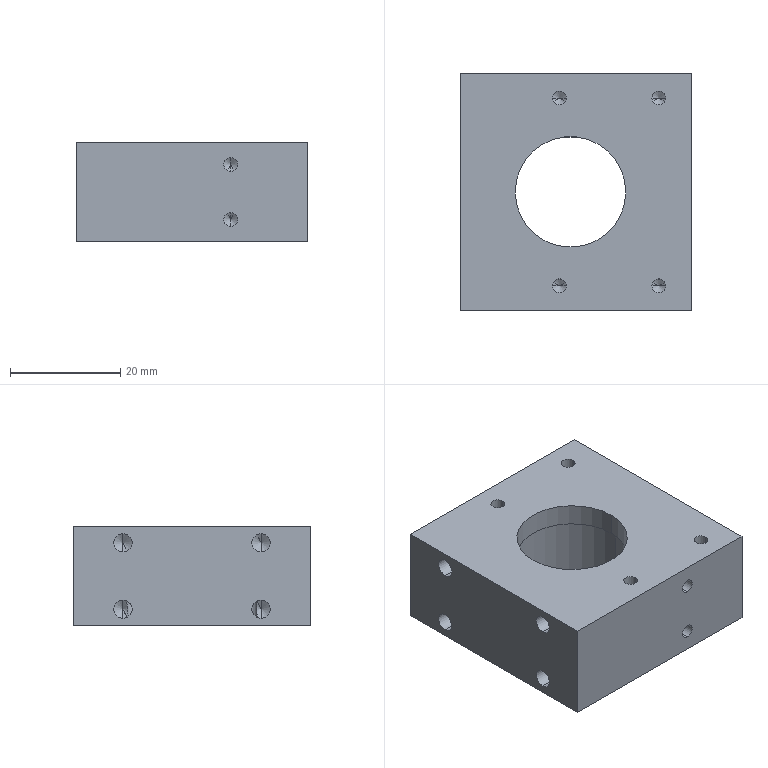Part | NX | features BREP 1 | 1 solid | 85 faces | box 42 x 43 x 18 mm | volume 24907 mm3 | cone 42 | cylinder 36 | plane 7 | commonest cylinder face diameters 2.5 x16 3.3 x16 20 x2 22 x2